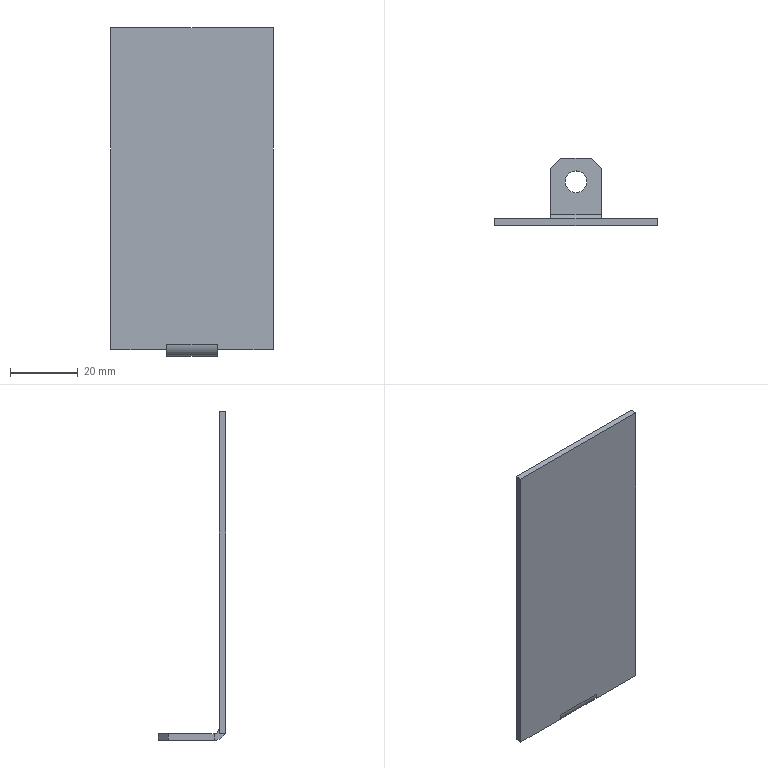Part | STEP file | Slide plate | 1 solid | 22 faces | box 48 x 20 x 97 mm | volume 9605 mm3 | plane 18 | cylinder 4 | commonest cylinder face diameters 6.4 x2 3 x1 7 x1